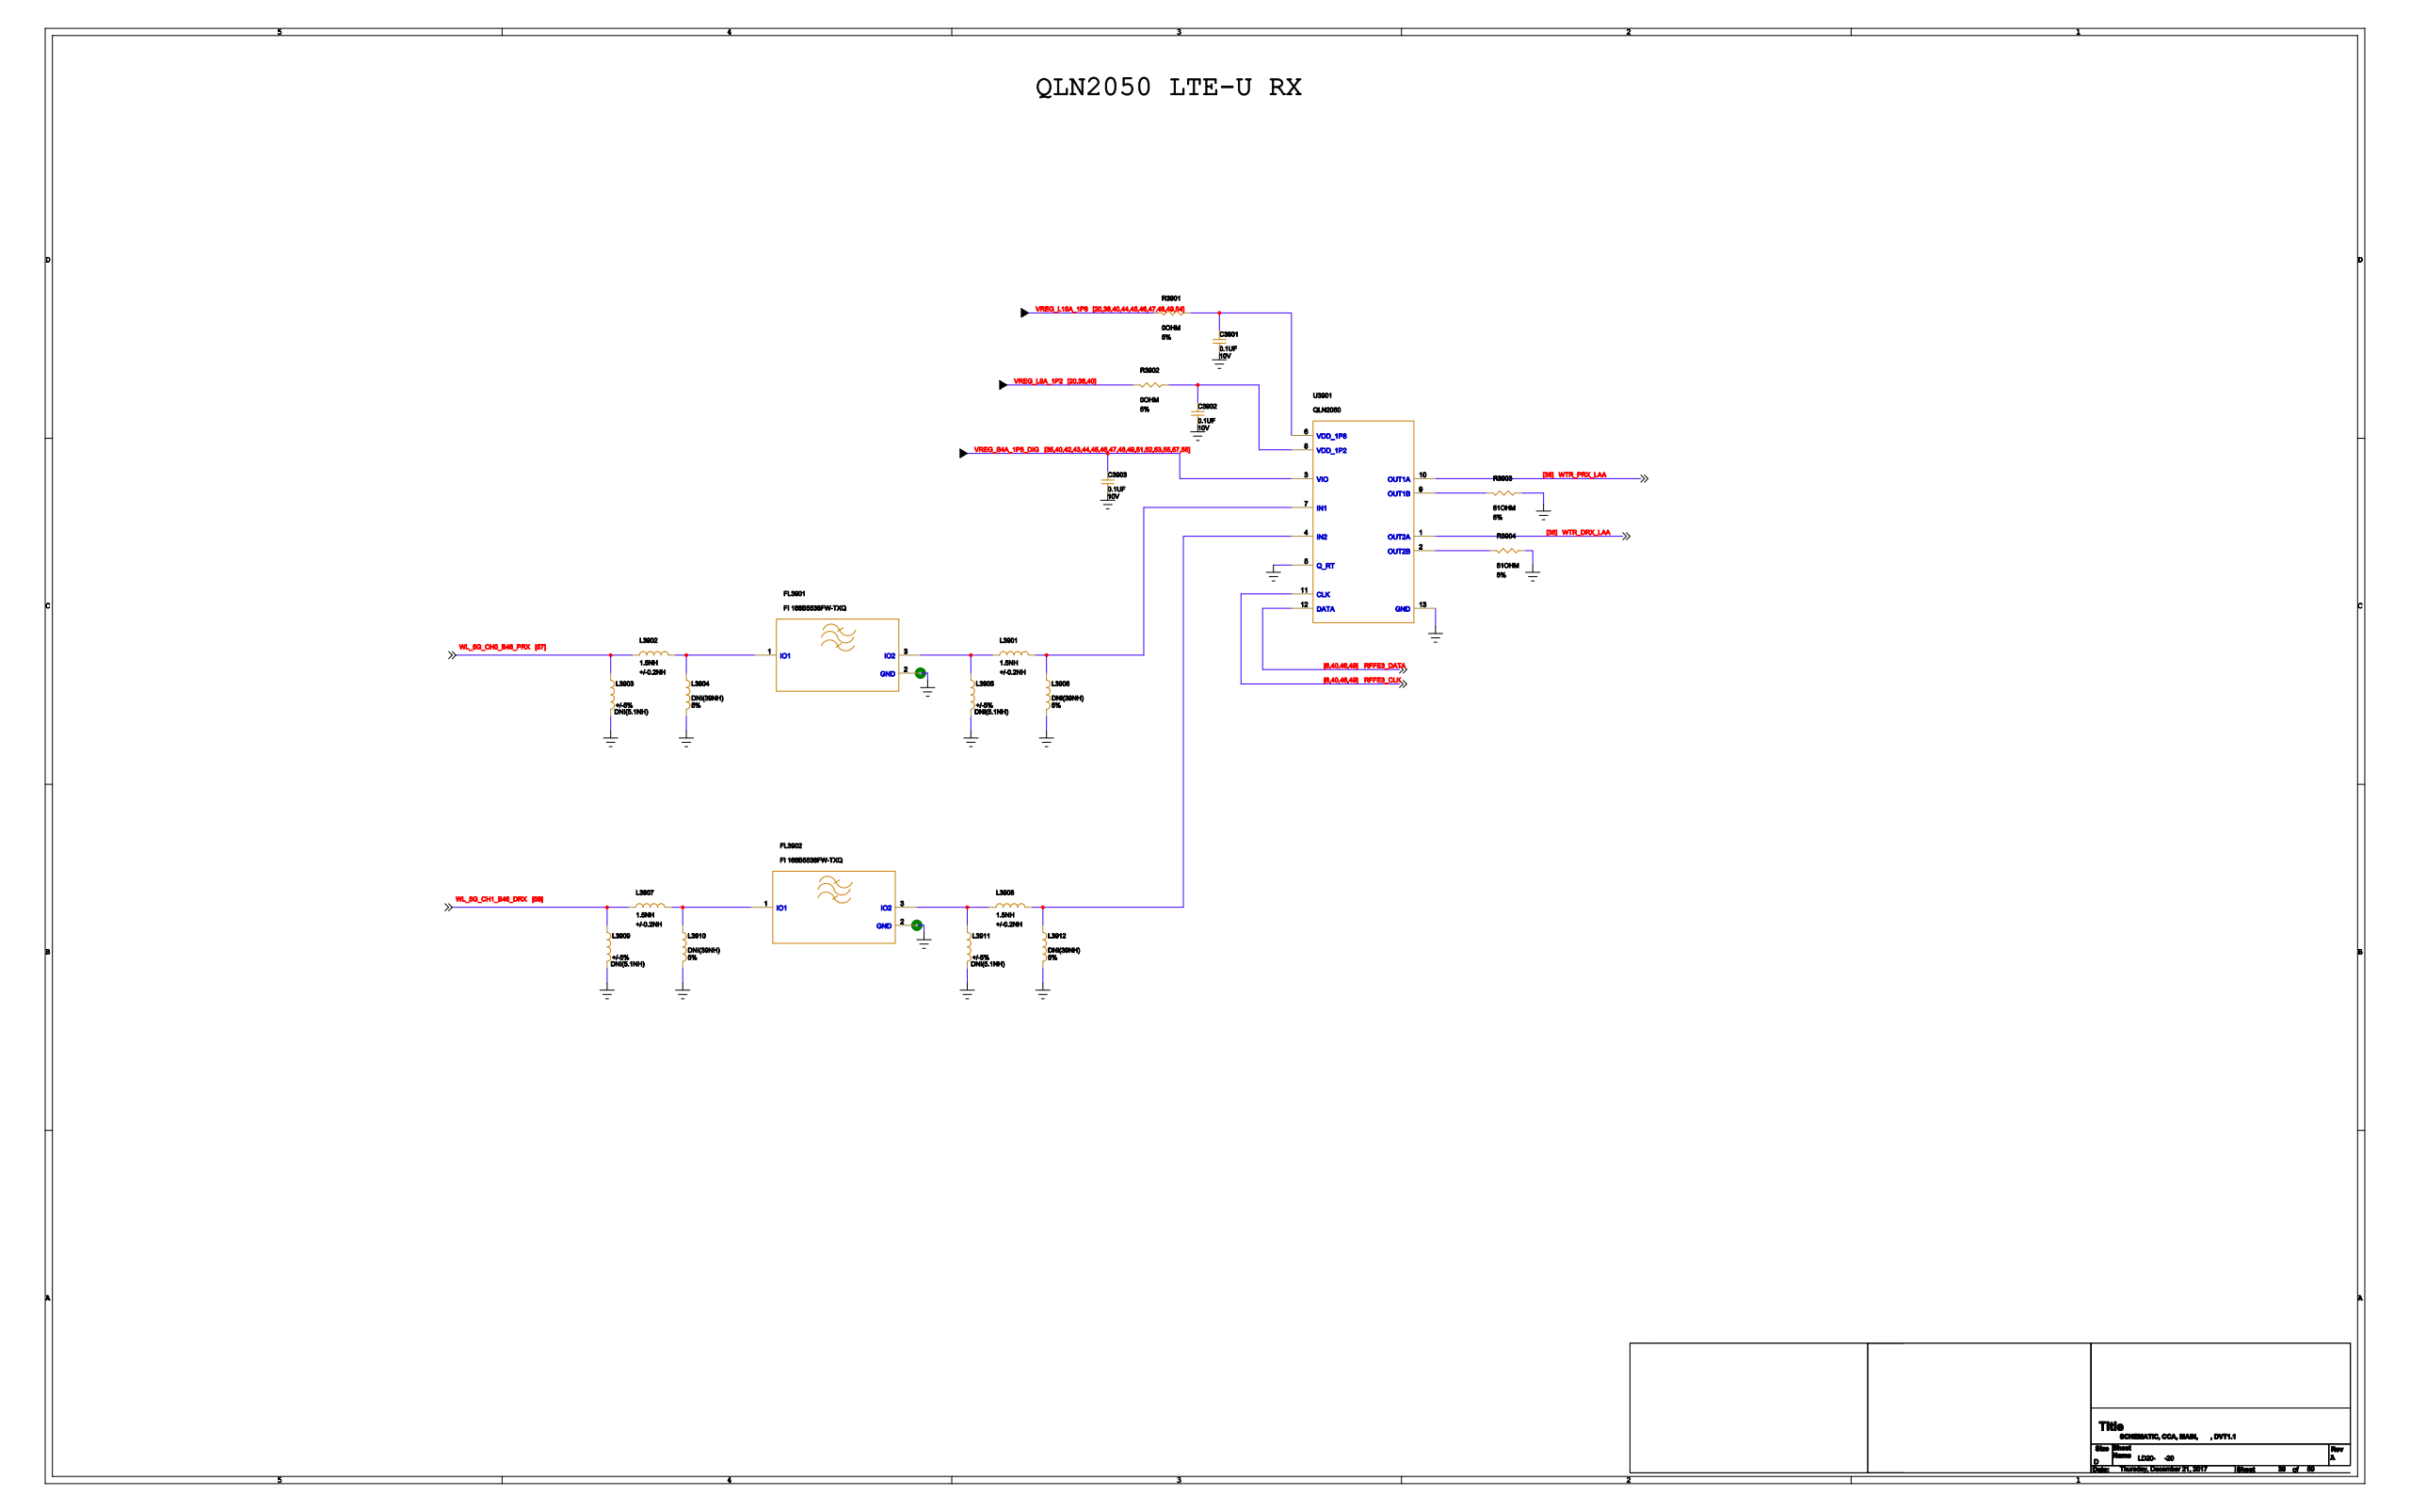Circuit board | Cadence Allegro | 1520 parts | 1149 nets | one sheet of the schematic
Parts on this sheet (reference | value | footprint):
C3901 | 0.1UF | 2P0201R
C3902 | 0.1UF | 2P0201R
C3903 | 0.1UF | 2P0201R
FL3901 | FI 168B5538FW-TXQ | 3PSM67X35NV2
FL3902 | FI 168B5538FW-TXQ | 3PSM67X35NV2
L3901 | 1.5NH | 2P0201R
L3902 | 1.5NH | 2P0201R
L3903 | DNI(5.1NH) | 2P0201R_DNI
L3904 | DNI(39NH) | 2P0201R_DNI
L3905 | DNI(5.1NH) | 2P0201R_DNI
L3906 | DNI(39NH) | 2P0201R_DNI
L3907 | 1.5NH | 2P0201R
L3908 | 1.5NH | 2P0201R
L3909 | DNI(5.1NH) | 2P0201R_DNI
L3910 | DNI(39NH) | 2P0201R_DNI
L3911 | DNI(5.1NH) | 2P0201R_DNI
L3912 | DNI(39NH) | 2P0201R_DNI
R3901 | 0OHM | 2P0201R
R3902 | 0OHM | 2P0201R
R3903 | 51OHM | 2P0201R
R3904 | 51OHM | 2P0201R
U3901 | QLN2050 | 13LGA79X81N
Nets of these parts (net: part-pin ...):
GND: C3901-2 C3902-2 C3903-2 FL3901-2 FL3902-2 L3903-2 L3904-2 L3905-2 L3906-2 L3909-2 L3910-2 L3911-2 L3912-2 R3903-2 R3904-2 U3901-5 U3901-13
VREG_L15A_1P8: R3901-1
WL_5G_CH0_B46_PRX: L3902-1 L3903-1
N48221875: FL3901-3 L3901-1 L3905-1
WL_5G_CH1_B46_DRX: L3907-1 L3909-1
N48222214: FL3902-3 L3908-1 L3911-1
N48221715: FL3901-1 L3902-2 L3904-1
N48221877: L3901-2 L3906-1 U3901-7
N48222160: FL3902-1 L3907-2 L3910-1
N48222212: L3908-2 L3912-1 U3901-4
VREG_S4A_1P8_DIG: C3903-1 U3901-3
VREG_L8A_1P2: R3902-1
WTR_DRX_LAA: U3901-1
WTR_PRX_LAA: U3901-10
RFFE3_CLK: U3901-11
RFFE3_DATA: U3901-12
N48221317: C3901-1 R3901-2 U3901-6
N48221248: C3902-1 R3902-2 U3901-8
N48222922: R3903-1 U3901-9
N48222794: R3904-1 U3901-2